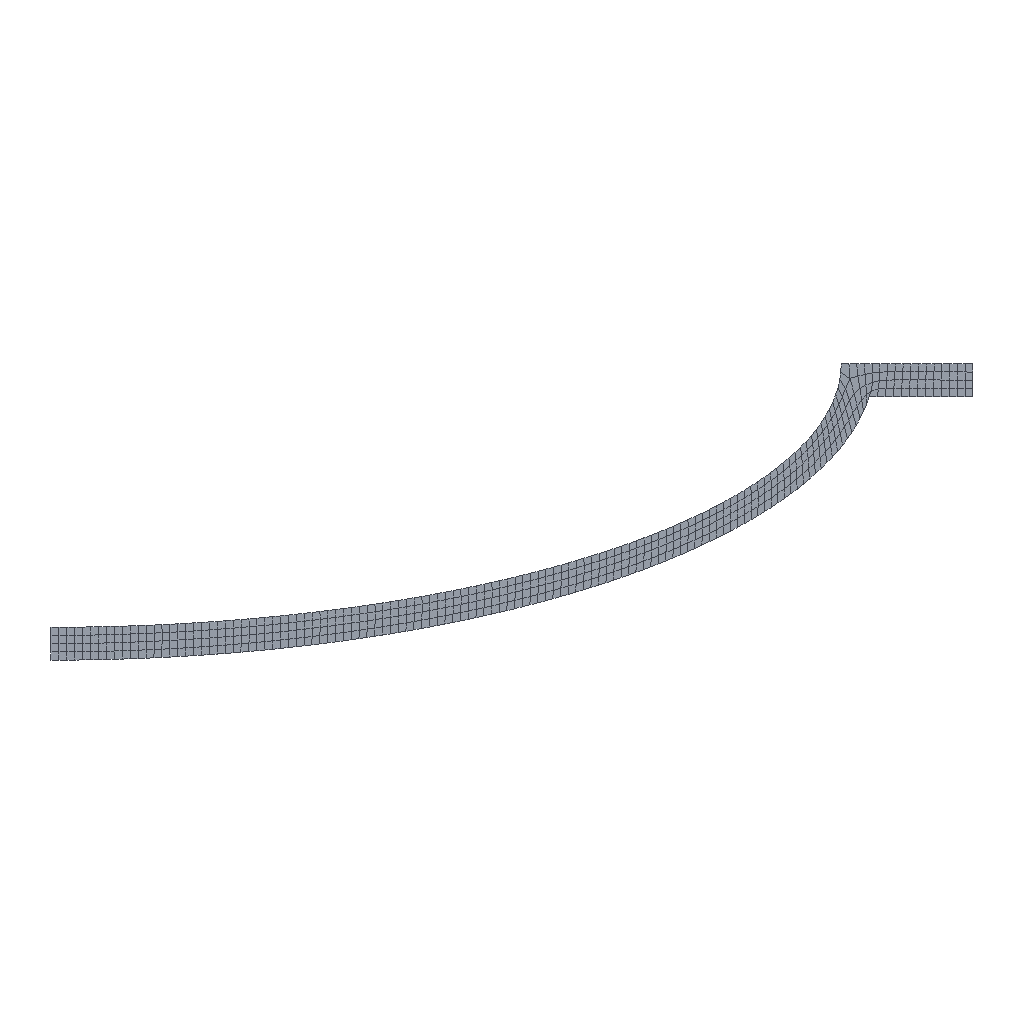Simulation study | abaqus
Set-up summary:
category,name,step,type,value,unit,region
solver,abaqus
solver,version,,,Abaqus/Standard 2020
units,not stated in the deck,,not stated
analysis,deck,,static,static
load_step,"""Static","""Static",static
load_step,requested,,,1
mesh,nodes,,,637
mesh,elements,,,505
element_type,CAX4H,,axisymmetric,505
load,load commands in deck,,count,1
bc,support commands in deck,,count,2
material,HYPERELASTIC,,in results
check,setup vs results,,match,"per instance, exact: element labels, types and connectivity; labels of the nodes the elements use; coordinates of those nodes at SINGLE_PRECISION in 1 of 1 instance(s)"
Abaqus input file, long lists of numbers shortened:
*Heading
** Job name: Job-1 Model name: gong
** Generated by: Abaqus/CAE 2020
*Preprint, echo=NO, model=NO, history=NO, contact=NO
**
** PARTS
**
*Part, name=gong2
*Node
      1,          35.,        -1.25
      2,          35.,      -0.3125
** (635 more lines like these left out)
*Element, type=CAX4H
  1,   1,  13, 390,  43
  2,  13,  14, 391, 390
** (503 more lines like these left out)
*Nset, nset=_PickedSet2, internal, generate
   1,  637,    1
*Elset, elset=_PickedSet2, internal, generate
   1,  505,    1
*Nset, nset=s1, generate
   1,  637,    1
*Nset, nset=s2
   5,  67,  68,  69,  70,  71,  72,  73,  74,  75,  76,  77,  78,  79,  80,  81
  82,  83,  84,  85,  86,  87,  88,  89,  90,  91,  92,  93,  94,  95,  96,  97
** (31 more lines like these left out)
** Section: gong2_section
*Solid Section, elset=_PickedSet2, material=hyperelastic
,
*End Part
**
**
** ASSEMBLY
**
*Assembly, name=Assembly
**
*Instance, name=gong2-1, part=gong2
*End Instance
**
*Nset, nset=_PickedSet14, internal, instance=gong2-1
  10,  11,  12, 279, 280
*Elset, elset=_PickedSet14, internal, instance=gong2-1, generate
 175,  178,    1
*Nset, nset=_PickedSet15, internal, instance=gong2-1
  6,  7,  8, 46, 47, 48, 49, 50, 51, 52, 53, 54, 55, 56, 57, 58
 59, 60
*Elset, elset=_PickedSet15, internal, instance=gong2-1, generate
 49,  65,   1
*Elset, elset=__PickedSurf21_S2, internal, instance=gong2-1
 65,
*Elset, elset=__PickedSurf21_S1, internal, instance=gong2-1, generate
  66,  175,    1
*Surface, type=ELEMENT, name=_PickedSurf21, internal
__PickedSurf21_S2, S2
__PickedSurf21_S1, S1
*End Assembly
**
** MATERIALS
**
*Material, name=hyperelastic
*Hyperelastic, neo hooke
 0.15, 0.001
**
** BOUNDARY CONDITIONS
**
** Name: BC-1 Type: 对称/反对称/完全固定
*Boundary
_PickedSet14, XSYMM
** Name: BC-2 Type: 对称/反对称/完全固定
*Boundary
_PickedSet15, ENCASTRE
** ----------------------------------------------------------------
**
** STEP: Static, Risks
**
*Step, name="Static, Risks", nlgeom=YES, inc=1000
*Static, riks
0.001, 1., 1e-05, 1., 0.8,
**
** LOADS
**
** Name: Load-2   Type: Pressure
*Dsload
_PickedSurf21, P, 0.019
**
** OUTPUT REQUESTS
**
*Restart, write, frequency=0
**
** FIELD OUTPUT: F-Output-2
**
*Output, field
*Node Output
CF, PHILSM, PSILSM, RF, RM, RT, TF, U
UR, UT, V, VF, VR, VT
*Element Output, directions=YES
ALPHA, ALPHAN, CFAILURE, CS11, CTSHR, DAMAGEC, DAMAGEFC, DAMAGEFT, DAMAGEMC, DAMAGEMT, DAMAGESHR, DAMAGET, DMICRT, E, ELEDEN, ELEN
ENER, ERPRATIO, ESF1, HSNFCCRT, HSNFTCRT, HSNMCCRT, HSNMTCRT, JK, MISES, MISESMAX, MISESONLY, NFORC, NFORCSO, P, PRESSONLY, PS
S, SDEG, SEQUT, SF, SHRRATIO, SSAVG, TRIAX, TSHR, VS, YIELDPOT
*Contact Output
BDSTAT, CRSTS, CSDMG, CSMAXSCRT, CSMAXUCRT, CSQUADSCRT, CSQUADUCRT, DBS, DBSF, DBT, EFENRRTR, ENRRT, OPENBC
**
** HISTORY OUTPUT: H-Output-2
**
*Output, history
*Element Output
IRA1, IRA2, IRA3, IRAR1, IRAR2, IRAR3, IRF1, IRF2, IRF3, IRM1, IRM2, IRM3
*Energy Output
ALLAE, ALLCD, ALLDMD, ALLEE, ALLFD, ALLIE, ALLJD, ALLKE, ALLKL, ALLPD, ALLQB, ALLSD, ALLSE, ALLVD, ALLWK, ETOTAL
*Contact Output
BDSTAT, CRSTS11, CRSTS12, CRSTS13, CSDMG, CSMAXSCRT, CSMAXUCRT, CSQUADSCRT, CSQUADUCRT, DBS11, DBS12, DBSF, DBT, EFENRRTR, ENRRT11, ENRRT12
ENRRT13, OPENBC
*End Step
Results summary:
result,step,,partial,increments=13 time=0.2585/1.0
result,analysis,,,"static, riks"
result,last_loadstep,,,1
result,primary field,,,U
result,reaction total,,FX,-5.962,model units
result,reaction total,,FY,51.829,model units
result,reaction total,,FZ,0.0,model units